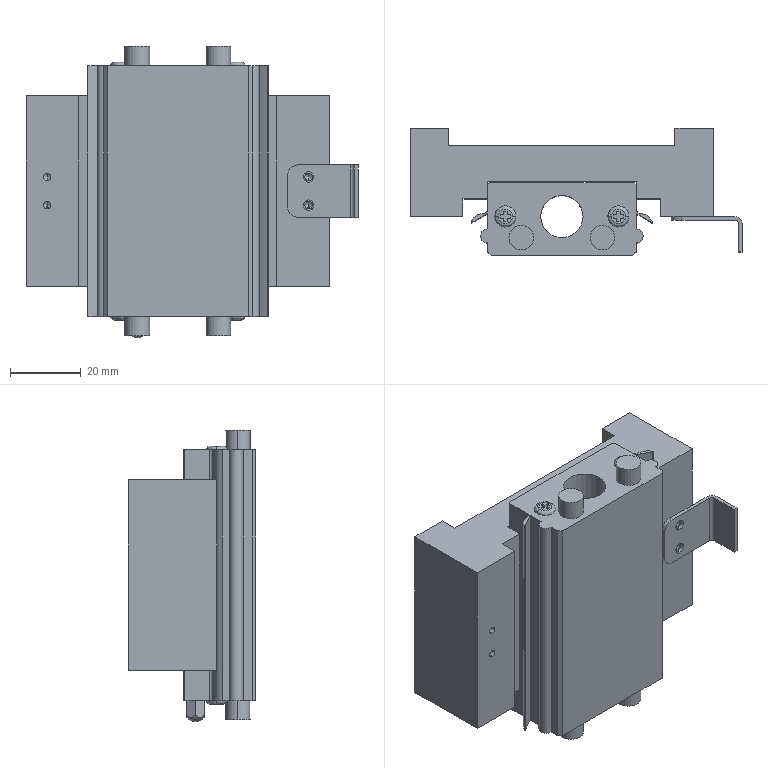Part | SolidWorks | features BaseBody 1 | 1 solid | 281 faces | box 94 x 36 x 82.5 mm | volume 126431 mm3 | plane 177 | cylinder 78 | cone 16 | spline 8 | torus 2 | commonest cylinder face diameters 2.113 x8 4.134 x8 5 x8 7 x8 9 x8 9.5 x8